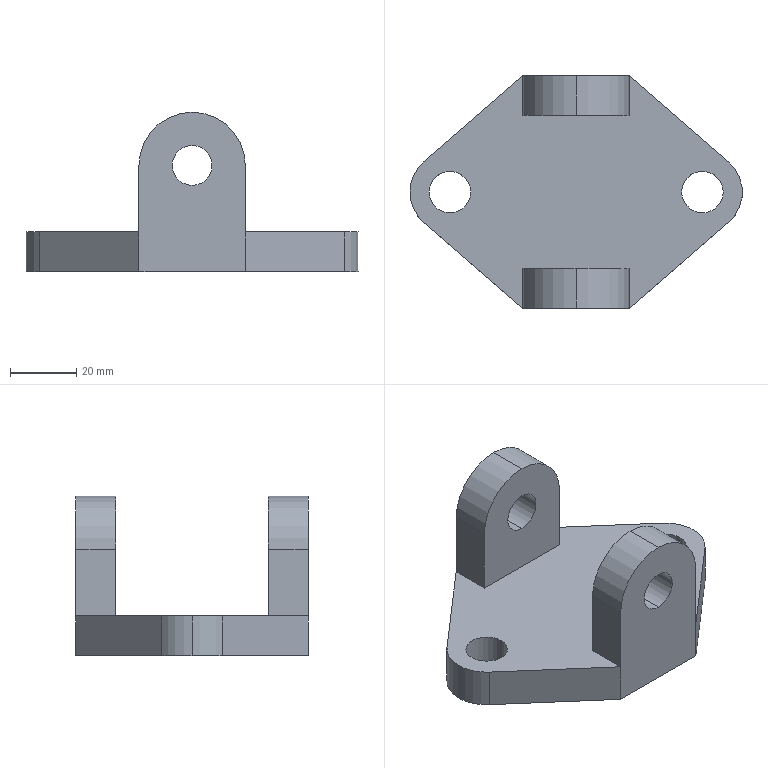Part | SolidWorks | features Cut 2, Boss 1, Extrusion 1, Fillet 1 | 1 solid | 29 faces | box 99.999 x 70 x 48 mm | volume 79061 mm3 | cylinder 15 | plane 14 | commonest cylinder face diameters 12 x4 12.5 x4 32 x4 24 x2 23.999 x1
STEP:
#1=CARTESIAN_POINT('',(0.,35.,38.));
#2=VERTEX_POINT('',#1);
#3=CARTESIAN_POINT('',(0.,35.,26.));
#4=VERTEX_POINT('',#3);
#5=CARTESIAN_POINT('',(0.,35.,32.));
#6=DIRECTION('',(0.,-1.,0.));
#7=DIRECTION('',(0.,0.,-1.));
#8=AXIS2_PLACEMENT_3D('',#5,#6,#7);
#9=CIRCLE('',#8,6.);
#10=EDGE_CURVE('',#2,#4,#9,.T.);
#11=ORIENTED_EDGE('',*,*,#10,.F.);
#12=CARTESIAN_POINT('',(0.,23.,38.));
#13=VERTEX_POINT('',#12);
#14=CARTESIAN_POINT('',(0.,43.,38.));
#15=DIRECTION('',(0.,-1.,0.));
#16=VECTOR('',#15,1000.);
#17=LINE('',#14,#16);
#18=EDGE_CURVE('',#2,#13,#17,.T.);
#19=ORIENTED_EDGE('',*,*,#18,.T.);
#20=CARTESIAN_POINT('',(0.,23.,26.));
#21=VERTEX_POINT('',#20);
#22=CARTESIAN_POINT('',(0.,23.,32.));
#23=DIRECTION('',(0.,1.,0.));
#24=DIRECTION('',(0.,0.,1.));
#25=AXIS2_PLACEMENT_3D('',#22,#23,#24);
#26=CIRCLE('',#25,6.);
#27=EDGE_CURVE('',#21,#13,#26,.T.);
#28=ORIENTED_EDGE('',*,*,#27,.F.);
#29=CARTESIAN_POINT('',(0.,43.,26.));
#30=DIRECTION('',(0.,-1.,0.));
#31=VECTOR('',#30,1000.);
#32=LINE('',#29,#31);
#33=EDGE_CURVE('',#4,#21,#32,.T.);
#34=ORIENTED_EDGE('',*,*,#33,.F.);
#35=EDGE_LOOP('',(#11,#19,#28,#34));
#36=FACE_OUTER_BOUND('',#35,.T.);
#37=CARTESIAN_POINT('',(0.,43.,32.));
#38=DIRECTION('',(0.,-1.,0.));
#39=DIRECTION('',(0.,0.,-1.));
#40=AXIS2_PLACEMENT_3D('',#37,#38,#39);
#41=CYLINDRICAL_SURFACE('',#40,6.);
#42=ADVANCED_FACE('',(#36),#41,.F.);
#43=CARTESIAN_POINT('',(0.,-23.,38.));
#44=VERTEX_POINT('',#43);
#45=CARTESIAN_POINT('',(0.,-23.,26.));
#46=VERTEX_POINT('',#45);
#47=CARTESIAN_POINT('',(0.,-23.,32.));
#48=DIRECTION('',(0.,-1.,0.));
#49=DIRECTION('',(0.,0.,-1.));
#50=AXIS2_PLACEMENT_3D('',#47,#48,#49);
#51=CIRCLE('',#50,6.);
#52=EDGE_CURVE('',#44,#46,#51,.T.);
#53=ORIENTED_EDGE('',*,*,#52,.F.);
#54=CARTESIAN_POINT('',(0.,-35.,38.));
#55=VERTEX_POINT('',#54);
#56=CARTESIAN_POINT('',(0.,43.,38.));
#57=DIRECTION('',(0.,-1.,0.));
#58=VECTOR('',#57,1000.);
#59=LINE('',#56,#58);
#60=EDGE_CURVE('',#44,#55,#59,.T.);
#61=ORIENTED_EDGE('',*,*,#60,.T.);
#62=CARTESIAN_POINT('',(0.,-35.,26.));
#63=VERTEX_POINT('',#62);
#64=CARTESIAN_POINT('',(0.,-35.,32.));
#65=DIRECTION('',(0.,-1.,0.));
#66=DIRECTION('',(0.,0.,-1.));
#67=AXIS2_PLACEMENT_3D('',#64,#65,#66);
#68=CIRCLE('',#67,6.);
#69=EDGE_CURVE('',#55,#63,#68,.T.);
#70=ORIENTED_EDGE('',*,*,#69,.T.);
#71=CARTESIAN_POINT('',(0.,43.,26.));
#72=DIRECTION('',(0.,-1.,0.));
#73=VECTOR('',#72,1000.);
#74=LINE('',#71,#73);
#75=EDGE_CURVE('',#46,#63,#74,.T.);
#76=ORIENTED_EDGE('',*,*,#75,.F.);
#77=EDGE_LOOP('',(#53,#61,#70,#76));
#78=FACE_OUTER_BOUND('',#77,.T.);
#79=CARTESIAN_POINT('',(0.,43.,32.));
#80=DIRECTION('',(0.,-1.,0.));
#81=DIRECTION('',(0.,0.,-1.));
#82=AXIS2_PLACEMENT_3D('',#79,#80,#81);
#83=CYLINDRICAL_SURFACE('',#82,6.);
#84=ADVANCED_FACE('',(#78),#83,.F.);
#85=CARTESIAN_POINT('',(31.75,0.,0.));
#86=VERTEX_POINT('',#85);
#87=CARTESIAN_POINT('',(44.25,0.,0.));
#88=VERTEX_POINT('',#87);
#89=CARTESIAN_POINT('',(38.,0.,0.));
#90=DIRECTION('',(0.,0.,1.));
#91=DIRECTION('',(1.,0.,0.));
#92=AXIS2_PLACEMENT_3D('',#89,#90,#91);
#93=CIRCLE('',#92,6.25);
#94=EDGE_CURVE('',#86,#88,#93,.T.);
#95=ORIENTED_EDGE('',*,*,#94,.F.);
#96=CARTESIAN_POINT('',(31.75,0.,12.));
#97=VERTEX_POINT('',#96);
#98=CARTESIAN_POINT('',(31.75,0.,0.));
#99=DIRECTION('',(0.,0.,1.));
#100=VECTOR('',#99,1000.);
#101=LINE('',#98,#100);
#102=EDGE_CURVE('',#86,#97,#101,.T.);
#103=ORIENTED_EDGE('',*,*,#102,.T.);
#104=CARTESIAN_POINT('',(44.25,0.,12.));
#105=VERTEX_POINT('',#104);
#106=CARTESIAN_POINT('',(38.,0.,12.));
#107=DIRECTION('',(0.,0.,1.));
#108=DIRECTION('',(1.,0.,0.));
#109=AXIS2_PLACEMENT_3D('',#106,#107,#108);
#110=CIRCLE('',#109,6.25);
#111=EDGE_CURVE('',#97,#105,#110,.T.);
#112=ORIENTED_EDGE('',*,*,#111,.T.);
#113=CARTESIAN_POINT('',(44.25,0.,0.));
#114=DIRECTION('',(0.,0.,1.));
#115=VECTOR('',#114,1000.);
#116=LINE('',#113,#115);
#117=EDGE_CURVE('',#88,#105,#116,.T.);
#118=ORIENTED_EDGE('',*,*,#117,.F.);
#119=EDGE_LOOP('',(#95,#103,#112,#118));
#120=FACE_OUTER_BOUND('',#119,.T.);
#121=CARTESIAN_POINT('',(38.,0.,0.));
#122=DIRECTION('',(0.,0.,1.));
#123=DIRECTION('',(1.,0.,0.));
#124=AXIS2_PLACEMENT_3D('',#121,#122,#123);
#125=CYLINDRICAL_SURFACE('',#124,6.25);
#126=ADVANCED_FACE('',(#120),#125,.F.);
#127=CARTESIAN_POINT('',(-44.25,0.,0.));
#128=VERTEX_POINT('',#127);
#129=CARTESIAN_POINT('',(-31.75,0.,0.));
#130=VERTEX_POINT('',#129);
#131=CARTESIAN_POINT('',(-38.,0.,0.));
#132=DIRECTION('',(0.,0.,1.));
#133=DIRECTION('',(1.,0.,0.));
#134=AXIS2_PLACEMENT_3D('',#131,#132,#133);
#135=CIRCLE('',#134,6.25);
#136=EDGE_CURVE('',#128,#130,#135,.T.);
#137=ORIENTED_EDGE('',*,*,#136,.F.);
#138=CARTESIAN_POINT('',(-44.25,0.,12.));
#139=VERTEX_POINT('',#138);
#140=CARTESIAN_POINT('',(-44.25,0.,0.));
#141=DIRECTION('',(0.,0.,1.));
#142=VECTOR('',#141,1000.);
#143=LINE('',#140,#142);
#144=EDGE_CURVE('',#128,#139,#143,.T.);
#145=ORIENTED_EDGE('',*,*,#144,.T.);
#146=CARTESIAN_POINT('',(-31.75,0.,12.));
#147=VERTEX_POINT('',#146);
#148=CARTESIAN_POINT('',(-38.,0.,12.));
#149=DIRECTION('',(0.,0.,1.));
#150=DIRECTION('',(1.,0.,0.));
#151=AXIS2_PLACEMENT_3D('',#148,#149,#150);
#152=CIRCLE('',#151,6.25);
#153=EDGE_CURVE('',#139,#147,#152,.T.);
#154=ORIENTED_EDGE('',*,*,#153,.T.);
#155=CARTESIAN_POINT('',(-31.75,0.,0.));
#156=DIRECTION('',(0.,0.,1.));
#157=VECTOR('',#156,1000.);
#158=LINE('',#155,#157);
#159=EDGE_CURVE('',#130,#147,#158,.T.);
#160=ORIENTED_EDGE('',*,*,#159,.F.);
#161=EDGE_LOOP('',(#137,#145,#154,#160));
#162=FACE_OUTER_BOUND('',#161,.T.);
#163=CARTESIAN_POINT('',(-38.,0.,0.));
#164=DIRECTION('',(0.,0.,1.));
#165=DIRECTION('',(1.,0.,0.));
#166=AXIS2_PLACEMENT_3D('',#163,#164,#165);
#167=CYLINDRICAL_SURFACE('',#166,6.25);
#168=ADVANCED_FACE('',(#162),#167,.F.);
#169=CARTESIAN_POINT('',(-50.,0.,12.));
#170=VERTEX_POINT('',#169);
#171=CARTESIAN_POINT('',(-45.868,-9.06,12.));
#172=VERTEX_POINT('',#171);
#173=CARTESIAN_POINT('',(-38.,0.,12.));
#174=DIRECTION('',(0.,0.,1.));
#175=DIRECTION('',(1.,0.,0.));
#176=AXIS2_PLACEMENT_3D('',#173,#174,#175);
#177=CIRCLE('',#176,12.);
#178=EDGE_CURVE('',#170,#172,#177,.T.);
#179=ORIENTED_EDGE('',*,*,#178,.F.);
#180=CARTESIAN_POINT('',(-50.,0.,0.));
#181=VERTEX_POINT('',#180);
#182=CARTESIAN_POINT('',(-50.,0.,12.));
#183=DIRECTION('',(0.,0.,-1.));
#184=VECTOR('',#183,1000.);
#185=LINE('',#182,#184);
#186=EDGE_CURVE('',#170,#181,#185,.T.);
#187=ORIENTED_EDGE('',*,*,#186,.T.);
#188=CARTESIAN_POINT('',(-45.868,-9.06,0.));
#189=VERTEX_POINT('',#188);
#190=CARTESIAN_POINT('',(-38.,0.,0.));
#191=DIRECTION('',(0.,0.,1.));
#192=DIRECTION('',(1.,0.,0.));
#193=AXIS2_PLACEMENT_3D('',#190,#191,#192);
#194=CIRCLE('',#193,12.);
#195=EDGE_CURVE('',#181,#189,#194,.T.);
#196=ORIENTED_EDGE('',*,*,#195,.T.);
#197=CARTESIAN_POINT('',(-45.868,-9.06,12.));
#198=DIRECTION('',(0.,0.,-1.));
#199=VECTOR('',#198,1000.);
#200=LINE('',#197,#199);
#201=EDGE_CURVE('',#172,#189,#200,.T.);
#202=ORIENTED_EDGE('',*,*,#201,.F.);
#203=EDGE_LOOP('',(#179,#187,#196,#202));
#204=FACE_OUTER_BOUND('',#203,.T.);
#205=CARTESIAN_POINT('',(-38.,0.,12.));
#206=DIRECTION('',(0.,0.,-1.));
#207=DIRECTION('',(-1.,0.,0.));
#208=AXIS2_PLACEMENT_3D('',#205,#206,#207);
#209=CYLINDRICAL_SURFACE('',#208,12.);
#210=ADVANCED_FACE('',(#204),#209,.T.);
#211=CARTESIAN_POINT('',(-38.,0.,12.));
#212=DIRECTION('',(0.,0.,1.));
#213=DIRECTION('',(1.,0.,0.));
#214=AXIS2_PLACEMENT_3D('',#211,#212,#213);
#215=CIRCLE('',#214,6.25);
#216=EDGE_CURVE('',#147,#139,#215,.T.);
#217=ORIENTED_EDGE('',*,*,#216,.F.);
#218=ORIENTED_EDGE('',*,*,#153,.F.);
#219=EDGE_LOOP('',(#217,#218));
#220=FACE_BOUND('',#219,.T.);
#221=CARTESIAN_POINT('',(38.,0.,12.));
#222=DIRECTION('',(0.,0.,1.));
#223=DIRECTION('',(1.,0.,0.));
#224=AXIS2_PLACEMENT_3D('',#221,#222,#223);
#225=CIRCLE('',#224,6.25);
#226=EDGE_CURVE('',#105,#97,#225,.T.);
#227=ORIENTED_EDGE('',*,*,#226,.F.);
#228=ORIENTED_EDGE('',*,*,#111,.F.);
#229=EDGE_LOOP('',(#227,#228));
#230=FACE_BOUND('',#229,.T.);
#231=CARTESIAN_POINT('',(-16.,-35.,12.));
#232=VERTEX_POINT('',#231);
#233=CARTESIAN_POINT('',(-16.,-35.,12.));
#234=DIRECTION('',(0.755,-0.6557,0.));
#235=VECTOR('',#234,1000.);
#236=LINE('',#233,#235);
#237=EDGE_CURVE('',#172,#232,#236,.T.);
#238=ORIENTED_EDGE('',*,*,#237,.T.);
#239=CARTESIAN_POINT('',(-16.,-23.,12.));
#240=VERTEX_POINT('',#239);
#241=CARTESIAN_POINT('',(-16.,-35.,12.));
#242=DIRECTION('',(0.,-1.,0.));
#243=VECTOR('',#242,1000.);
#244=LINE('',#241,#243);
#245=EDGE_CURVE('',#240,#232,#244,.T.);
#246=ORIENTED_EDGE('',*,*,#245,.F.);
#247=CARTESIAN_POINT('',(16.,-23.,12.));
#248=VERTEX_POINT('',#247);
#249=CARTESIAN_POINT('',(-16.,-23.,12.));
#250=DIRECTION('',(-1.,0.,0.));
#251=VECTOR('',#250,1000.);
#252=LINE('',#249,#251);
#253=EDGE_CURVE('',#248,#240,#252,.T.);
#254=ORIENTED_EDGE('',*,*,#253,.F.);
#255=CARTESIAN_POINT('',(16.,-35.,12.));
#256=VERTEX_POINT('',#255);
#257=CARTESIAN_POINT('',(16.,-35.,12.));
#258=DIRECTION('',(0.,1.,0.));
#259=VECTOR('',#258,1000.);
#260=LINE('',#257,#259);
#261=EDGE_CURVE('',#256,#248,#260,.T.);
#262=ORIENTED_EDGE('',*,*,#261,.F.);
#263=CARTESIAN_POINT('',(45.868,-9.06,12.));
#264=VERTEX_POINT('',#263);
#265=CARTESIAN_POINT('',(16.,-35.,12.));
#266=DIRECTION('',(0.755,0.6557,0.));
#267=VECTOR('',#266,1000.);
#268=LINE('',#265,#267);
#269=EDGE_CURVE('',#256,#264,#268,.T.);
#270=ORIENTED_EDGE('',*,*,#269,.T.);
#271=CARTESIAN_POINT('',(45.868,9.06,12.));
#272=VERTEX_POINT('',#271);
#273=CARTESIAN_POINT('',(38.,0.,12.));
#274=DIRECTION('',(0.,0.,1.));
#275=DIRECTION('',(1.,0.,0.));
#276=AXIS2_PLACEMENT_3D('',#273,#274,#275);
#277=CIRCLE('',#276,11.999);
#278=EDGE_CURVE('',#264,#272,#277,.T.);
#279=ORIENTED_EDGE('',*,*,#278,.T.);
#280=CARTESIAN_POINT('',(16.,35.,12.));
#281=VERTEX_POINT('',#280);
#282=CARTESIAN_POINT('',(16.,35.,12.));
#283=DIRECTION('',(-0.755,0.6557,0.));
#284=VECTOR('',#283,1000.);
#285=LINE('',#282,#284);
#286=EDGE_CURVE('',#272,#281,#285,.T.);
#287=ORIENTED_EDGE('',*,*,#286,.T.);
#288=CARTESIAN_POINT('',(16.,23.,12.));
#289=VERTEX_POINT('',#288);
#290=CARTESIAN_POINT('',(16.,35.,12.));
#291=DIRECTION('',(0.,1.,0.));
#292=VECTOR('',#291,1000.);
#293=LINE('',#290,#292);
#294=EDGE_CURVE('',#289,#281,#293,.T.);
#295=ORIENTED_EDGE('',*,*,#294,.F.);
#296=CARTESIAN_POINT('',(-16.,23.,12.));
#297=VERTEX_POINT('',#296);
#298=CARTESIAN_POINT('',(-16.,23.,12.));
#299=DIRECTION('',(1.,0.,0.));
#300=VECTOR('',#299,1000.);
#301=LINE('',#298,#300);
#302=EDGE_CURVE('',#297,#289,#301,.T.);
#303=ORIENTED_EDGE('',*,*,#302,.F.);
#304=CARTESIAN_POINT('',(-16.,35.,12.));
#305=VERTEX_POINT('',#304);
#306=CARTESIAN_POINT('',(-16.,35.,12.));
#307=DIRECTION('',(0.,-1.,0.));
#308=VECTOR('',#307,1000.);
#309=LINE('',#306,#308);
#310=EDGE_CURVE('',#305,#297,#309,.T.);
#311=ORIENTED_EDGE('',*,*,#310,.F.);
#312=CARTESIAN_POINT('',(-45.868,9.06,12.));
#313=VERTEX_POINT('',#312);
#314=CARTESIAN_POINT('',(-16.,35.,12.));
#315=DIRECTION('',(-0.755,-0.6557,0.));
#316=VECTOR('',#315,1000.);
#317=LINE('',#314,#316);
#318=EDGE_CURVE('',#305,#313,#317,.T.);
#319=ORIENTED_EDGE('',*,*,#318,.T.);
#320=CARTESIAN_POINT('',(-38.,0.,12.));
#321=DIRECTION('',(0.,0.,1.));
#322=DIRECTION('',(1.,0.,0.));
#323=AXIS2_PLACEMENT_3D('',#320,#321,#322);
#324=CIRCLE('',#323,12.);
#325=EDGE_CURVE('',#313,#170,#324,.T.);
#326=ORIENTED_EDGE('',*,*,#325,.T.);
#327=ORIENTED_EDGE('',*,*,#178,.T.);
#328=EDGE_LOOP('',(#238,#246,#254,#262,#270,#279,#287,#295,#303,#311,#319,#326,#327));
#329=FACE_OUTER_BOUND('',#328,.T.);
#330=CARTESIAN_POINT('',(38.,0.,12.));
#331=DIRECTION('',(0.,0.,1.));
#332=DIRECTION('',(1.,0.,0.));
#333=AXIS2_PLACEMENT_3D('',#330,#331,#332);
#334=PLANE('',#333);
#335=ADVANCED_FACE('',(#220,#230,#329),#334,.T.);
#336=CARTESIAN_POINT('',(0.,35.,32.));
#337=DIRECTION('',(0.,-1.,0.));
#338=DIRECTION('',(0.,0.,-1.));
#339=AXIS2_PLACEMENT_3D('',#336,#337,#338);
#340=CIRCLE('',#339,6.);
#341=EDGE_CURVE('',#4,#2,#340,.T.);
#342=ORIENTED_EDGE('',*,*,#341,.T.);
#343=ORIENTED_EDGE('',*,*,#10,.T.);
#344=EDGE_LOOP('',(#342,#343));
#345=FACE_BOUND('',#344,.T.);
#346=CARTESIAN_POINT('',(-16.,35.,32.));
#347=VERTEX_POINT('',#346);
#348=CARTESIAN_POINT('',(0.,35.,48.));
#349=VERTEX_POINT('',#348);
#350=CARTESIAN_POINT('',(0.,35.,32.));
#351=DIRECTION('',(0.,1.,0.));
#352=DIRECTION('',(0.,0.,-1.));
#353=AXIS2_PLACEMENT_3D('',#350,#351,#352);
#354=CIRCLE('',#353,16.);
#355=EDGE_CURVE('',#347,#349,#354,.T.);
#356=ORIENTED_EDGE('',*,*,#355,.T.);
#357=CARTESIAN_POINT('',(16.,35.,32.));
#358=VERTEX_POINT('',#357);
#359=CARTESIAN_POINT('',(0.,35.,32.));
#360=DIRECTION('',(0.,1.,0.));
#361=DIRECTION('',(0.,0.,-1.));
#362=AXIS2_PLACEMENT_3D('',#359,#360,#361);
#363=CIRCLE('',#362,16.);
#364=EDGE_CURVE('',#349,#358,#363,.T.);
#365=ORIENTED_EDGE('',*,*,#364,.T.);
#366=CARTESIAN_POINT('',(16.,35.,48.));
#367=DIRECTION('',(0.,0.,-1.));
#368=VECTOR('',#367,1000.);
#369=LINE('',#366,#368);
#370=EDGE_CURVE('',#358,#281,#369,.T.);
#371=ORIENTED_EDGE('',*,*,#370,.T.);
#372=CARTESIAN_POINT('',(16.,35.,0.));
#373=VERTEX_POINT('',#372);
#374=CARTESIAN_POINT('',(16.,35.,12.));
#375=DIRECTION('',(0.,0.,-1.));
#376=VECTOR('',#375,1000.);
#377=LINE('',#374,#376);
#378=EDGE_CURVE('',#281,#373,#377,.T.);
#379=ORIENTED_EDGE('',*,*,#378,.T.);
#380=CARTESIAN_POINT('',(-16.,35.,0.));
#381=VERTEX_POINT('',#380);
#382=CARTESIAN_POINT('',(0.,35.,0.));
#383=DIRECTION('',(-1.,0.,0.));
#384=VECTOR('',#383,1000.);
#385=LINE('',#382,#384);
#386=EDGE_CURVE('',#373,#381,#385,.T.);
#387=ORIENTED_EDGE('',*,*,#386,.T.);
#388=CARTESIAN_POINT('',(-16.,35.,12.));
#389=DIRECTION('',(0.,0.,-1.));
#390=VECTOR('',#389,1000.);
#391=LINE('',#388,#390);
#392=EDGE_CURVE('',#305,#381,#391,.T.);
#393=ORIENTED_EDGE('',*,*,#392,.F.);
#394=CARTESIAN_POINT('',(-16.,35.,48.));
#395=DIRECTION('',(0.,0.,-1.));
#396=VECTOR('',#395,1000.);
#397=LINE('',#394,#396);
#398=EDGE_CURVE('',#347,#305,#397,.T.);
#399=ORIENTED_EDGE('',*,*,#398,.F.);
#400=EDGE_LOOP('',(#356,#365,#371,#379,#387,#393,#399));
#401=FACE_OUTER_BOUND('',#400,.T.);
#402=CARTESIAN_POINT('',(0.,35.,12.));
#403=DIRECTION('',(0.,-1.,0.));
#404=DIRECTION('',(0.,0.,-1.));
#405=AXIS2_PLACEMENT_3D('',#402,#403,#404);
#406=PLANE('',#405);
#407=ADVANCED_FACE('',(#345,#401),#406,.F.);
#408=CARTESIAN_POINT('',(-45.868,9.06,0.));
#409=VERTEX_POINT('',#408);
#410=CARTESIAN_POINT('',(-16.,35.,0.));
#411=DIRECTION('',(-0.755,-0.6557,0.));
#412=VECTOR('',#411,1000.);
#413=LINE('',#410,#412);
#414=EDGE_CURVE('',#381,#409,#413,.T.);
#415=ORIENTED_EDGE('',*,*,#414,.T.);
#416=CARTESIAN_POINT('',(-45.868,9.06,12.));
#417=DIRECTION('',(0.,0.,-1.));
#418=VECTOR('',#417,1000.);
#419=LINE('',#416,#418);
#420=EDGE_CURVE('',#313,#409,#419,.T.);
#421=ORIENTED_EDGE('',*,*,#420,.F.);
#422=ORIENTED_EDGE('',*,*,#318,.F.);
#423=ORIENTED_EDGE('',*,*,#392,.T.);
#424=EDGE_LOOP('',(#415,#421,#422,#423));
#425=FACE_OUTER_BOUND('',#424,.T.);
#426=CARTESIAN_POINT('',(-16.,35.,12.));
#427=DIRECTION('',(0.6557,-0.755,0.));
#428=DIRECTION('',(0.755,0.6557,0.));
#429=AXIS2_PLACEMENT_3D('',#426,#427,#428);
#430=PLANE('',#429);
#431=ADVANCED_FACE('',(#425),#430,.F.);
#432=ORIENTED_EDGE('',*,*,#186,.F.);
#433=ORIENTED_EDGE('',*,*,#325,.F.);
#434=ORIENTED_EDGE('',*,*,#420,.T.);
#435=CARTESIAN_POINT('',(-38.,0.,0.));
#436=DIRECTION('',(0.,0.,1.));
#437=DIRECTION('',(1.,0.,0.));
#438=AXIS2_PLACEMENT_3D('',#435,#436,#437);
#439=CIRCLE('',#438,12.);
#440=EDGE_CURVE('',#409,#181,#439,.T.);
#441=ORIENTED_EDGE('',*,*,#440,.T.);
#442=EDGE_LOOP('',(#432,#433,#434,#441));
#443=FACE_OUTER_BOUND('',#442,.T.);
#444=CARTESIAN_POINT('',(-38.,0.,12.));
#445=DIRECTION('',(0.,0.,-1.));
#446=DIRECTION('',(-1.,0.,0.));
#447=AXIS2_PLACEMENT_3D('',#444,#445,#446);
#448=CYLINDRICAL_SURFACE('',#447,12.);
#449=ADVANCED_FACE('',(#443),#448,.T.);
#450=CARTESIAN_POINT('',(-16.,-35.,0.));
#451=VERTEX_POINT('',#450);
#452=CARTESIAN_POINT('',(-16.,-35.,0.));
#453=DIRECTION('',(0.755,-0.6557,0.));
#454=VECTOR('',#453,1000.);
#455=LINE('',#452,#454);
#456=EDGE_CURVE('',#189,#451,#455,.T.);
#457=ORIENTED_EDGE('',*,*,#456,.T.);
#458=CARTESIAN_POINT('',(-16.,-35.,12.));
#459=DIRECTION('',(0.,0.,-1.));
#460=VECTOR('',#459,1000.);
#461=LINE('',#458,#460);
#462=EDGE_CURVE('',#232,#451,#461,.T.);
#463=ORIENTED_EDGE('',*,*,#462,.F.);
#464=ORIENTED_EDGE('',*,*,#237,.F.);
#465=ORIENTED_EDGE('',*,*,#201,.T.);
#466=EDGE_LOOP('',(#457,#463,#464,#465));
#467=FACE_OUTER_BOUND('',#466,.T.);
#468=CARTESIAN_POINT('',(-16.,-35.,12.));
#469=DIRECTION('',(0.6557,0.755,0.));
#470=DIRECTION('',(-0.755,0.6557,0.));
#471=AXIS2_PLACEMENT_3D('',#468,#469,#470);
#472=PLANE('',#471);
#473=ADVANCED_FACE('',(#467),#472,.F.);
#474=CARTESIAN_POINT('',(0.,-35.,32.));
#475=DIRECTION('',(0.,-1.,0.));
#476=DIRECTION('',(0.,0.,-1.));
#477=AXIS2_PLACEMENT_3D('',#474,#475,#476);
#478=CIRCLE('',#477,6.);
#479=EDGE_CURVE('',#63,#55,#478,.T.);
#480=ORIENTED_EDGE('',*,*,#479,.F.);
#481=ORIENTED_EDGE('',*,*,#69,.F.);
#482=EDGE_LOOP('',(#480,#481));
#483=FACE_BOUND('',#482,.T.);
#484=CARTESIAN_POINT('',(16.,-35.,32.));
#485=VERTEX_POINT('',#484);
#486=CARTESIAN_POINT('',(16.,-35.,48.));
#487=DIRECTION('',(0.,0.,-1.));
#488=VECTOR('',#487,1000.);
#489=LINE('',#486,#488);
#490=EDGE_CURVE('',#485,#256,#489,.T.);
#491=ORIENTED_EDGE('',*,*,#490,.F.);
#492=CARTESIAN_POINT('',(0.,-35.,48.));
#493=VERTEX_POINT('',#492);
#494=CARTESIAN_POINT('',(0.,-35.,32.));
#495=DIRECTION('',(0.,-1.,0.));
#496=DIRECTION('',(0.,0.,1.));
#497=AXIS2_PLACEMENT_3D('',#494,#495,#496);
#498=CIRCLE('',#497,16.);
#499=EDGE_CURVE('',#485,#493,#498,.T.);
#500=ORIENTED_EDGE('',*,*,#499,.T.);
#501=CARTESIAN_POINT('',(-16.,-35.,32.));
#502=VERTEX_POINT('',#501);
#503=CARTESIAN_POINT('',(0.,-35.,32.));
#504=DIRECTION('',(0.,-1.,0.));
#505=DIRECTION('',(0.,0.,1.));
#506=AXIS2_PLACEMENT_3D('',#503,#504,#505);
#507=CIRCLE('',#506,16.);
#508=EDGE_CURVE('',#493,#502,#507,.T.);
#509=ORIENTED_EDGE('',*,*,#508,.T.);
#510=CARTESIAN_POINT('',(-16.,-35.,48.));
#511=DIRECTION('',(0.,0.,-1.));
#512=VECTOR('',#511,1000.);
#513=LINE('',#510,#512);
#514=EDGE_CURVE('',#502,#232,#513,.T.);
#515=ORIENTED_EDGE('',*,*,#514,.T.);
#516=ORIENTED_EDGE('',*,*,#462,.T.);
#517=CARTESIAN_POINT('',(16.,-35.,0.));
#518=VERTEX_POINT('',#517);
#519=CARTESIAN_POINT('',(-16.,-35.,0.));
#520=DIRECTION('',(1.,0.,0.));
#521=VECTOR('',#520,1000.);
#522=LINE('',#519,#521);
#523=EDGE_CURVE('',#451,#518,#522,.T.);
#524=ORIENTED_EDGE('',*,*,#523,.T.);
#525=CARTESIAN_POINT('',(16.,-35.,12.));
#526=DIRECTION('',(0.,0.,-1.));
#527=VECTOR('',#526,1000.);
#528=LINE('',#525,#527);
#529=EDGE_CURVE('',#256,#518,#528,.T.);
#530=ORIENTED_EDGE('',*,*,#529,.F.);
#531=EDGE_LOOP('',(#491,#500,#509,#515,#516,#524,#530));
#532=FACE_OUTER_BOUND('',#531,.T.);
#533=CARTESIAN_POINT('',(-16.,-35.,12.));
#534=DIRECTION('',(0.,1.,0.));
#535=DIRECTION('',(0.,0.,1.));
#536=AXIS2_PLACEMENT_3D('',#533,#534,#535);
#537=PLANE('',#536);
#538=ADVANCED_FACE('',(#483,#532),#537,.F.);
#539=CARTESIAN_POINT('',(45.868,-9.06,0.));
#540=VERTEX_POINT('',#539);
#541=CARTESIAN_POINT('',(16.,-35.,0.));
#542=DIRECTION('',(0.755,0.6557,0.));
#543=VECTOR('',#542,1000.);
#544=LINE('',#541,#543);
#545=EDGE_CURVE('',#518,#540,#544,.T.);
#546=ORIENTED_EDGE('',*,*,#545,.T.);
#547=CARTESIAN_POINT('',(45.868,-9.06,12.));
#548=DIRECTION('',(0.,0.,-1.));
#549=VECTOR('',#548,1000.);
#550=LINE('',#547,#549);
#551=EDGE_CURVE('',#264,#540,#550,.T.);
#552=ORIENTED_EDGE('',*,*,#551,.F.);
#553=ORIENTED_EDGE('',*,*,#269,.F.);
#554=ORIENTED_EDGE('',*,*,#529,.T.);
#555=EDGE_LOOP('',(#546,#552,#553,#554));
#556=FACE_OUTER_BOUND('',#555,.T.);
#557=CARTESIAN_POINT('',(16.,-35.,12.));
#558=DIRECTION('',(-0.6557,0.755,0.));
#559=DIRECTION('',(-0.755,-0.6557,0.));
#560=AXIS2_PLACEMENT_3D('',#557,#558,#559);
#561=PLANE('',#560);
#562=ADVANCED_FACE('',(#556),#561,.F.);
#563=CARTESIAN_POINT('',(45.868,9.06,0.));
#564=VERTEX_POINT('',#563);
#565=CARTESIAN_POINT('',(38.,0.,0.));
#566=DIRECTION('',(0.,0.,1.));
#567=DIRECTION('',(1.,0.,0.));
#568=AXIS2_PLACEMENT_3D('',#565,#566,#567);
#569=CIRCLE('',#568,11.999);
#570=EDGE_CURVE('',#540,#564,#569,.T.);
#571=ORIENTED_EDGE('',*,*,#570,.T.);
#572=CARTESIAN_POINT('',(45.868,9.06,12.));
#573=DIRECTION('',(0.,0.,-1.));
#574=VECTOR('',#573,1000.);
#575=LINE('',#572,#574);
#576=EDGE_CURVE('',#272,#564,#575,.T.);
#577=ORIENTED_EDGE('',*,*,#576,.F.);
#578=ORIENTED_EDGE('',*,*,#278,.F.);
#579=ORIENTED_EDGE('',*,*,#551,.T.);
#580=EDGE_LOOP('',(#571,#577,#578,#579));
#581=FACE_OUTER_BOUND('',#580,.T.);
#582=CARTESIAN_POINT('',(38.,0.,12.));
#583=DIRECTION('',(0.,0.,-1.));
#584=DIRECTION('',(-1.,0.,0.));
#585=AXIS2_PLACEMENT_3D('',#582,#583,#584);
#586=CYLINDRICAL_SURFACE('',#585,11.999);
#587=ADVANCED_FACE('',(#581),#586,.T.);
#588=CARTESIAN_POINT('',(16.,35.,0.));
#589=DIRECTION('',(-0.755,0.6557,0.));
#590=VECTOR('',#589,1000.);
#591=LINE('',#588,#590);
#592=EDGE_CURVE('',#564,#373,#591,.T.);
#593=ORIENTED_EDGE('',*,*,#592,.T.);
#594=ORIENTED_EDGE('',*,*,#378,.F.);
#595=ORIENTED_EDGE('',*,*,#286,.F.);
#596=ORIENTED_EDGE('',*,*,#576,.T.);
#597=EDGE_LOOP('',(#593,#594,#595,#596));
#598=FACE_OUTER_BOUND('',#597,.T.);
#599=CARTESIAN_POINT('',(16.,35.,12.));
#600=DIRECTION('',(-0.6557,-0.755,0.));
#601=DIRECTION('',(0.755,-0.6557,0.));
#602=AXIS2_PLACEMENT_3D('',#599,#600,#601);
#603=PLANE('',#602);
#604=ADVANCED_FACE('',(#598),#603,.F.);
#605=CARTESIAN_POINT('',(38.,0.,0.));
#606=DIRECTION('',(0.,0.,1.));
#607=DIRECTION('',(1.,0.,0.));
#608=AXIS2_PLACEMENT_3D('',#605,#606,#607);
#609=CIRCLE('',#608,6.25);
#610=EDGE_CURVE('',#88,#86,#609,.T.);
#611=ORIENTED_EDGE('',*,*,#610,.T.);
#612=ORIENTED_EDGE('',*,*,#94,.T.);
#613=EDGE_LOOP('',(#611,#612));
#614=FACE_BOUND('',#613,.T.);
#615=CARTESIAN_POINT('',(-38.,0.,0.));
#616=DIRECTION('',(0.,0.,1.));
#617=DIRECTION('',(1.,0.,0.));
#618=AXIS2_PLACEMENT_3D('',#615,#616,#617);
#619=CIRCLE('',#618,6.25);
#620=EDGE_CURVE('',#130,#128,#619,.T.);
#621=ORIENTED_EDGE('',*,*,#620,.T.);
#622=ORIENTED_EDGE('',*,*,#136,.T.);
#623=EDGE_LOOP('',(#621,#622));
#624=FACE_BOUND('',#623,.T.);
#625=ORIENTED_EDGE('',*,*,#386,.F.);
#626=ORIENTED_EDGE('',*,*,#592,.F.);
#627=ORIENTED_EDGE('',*,*,#570,.F.);
#628=ORIENTED_EDGE('',*,*,#545,.F.);
#629=ORIENTED_EDGE('',*,*,#523,.F.);
#630=ORIENTED_EDGE('',*,*,#456,.F.);
#631=ORIENTED_EDGE('',*,*,#195,.F.);
#632=ORIENTED_EDGE('',*,*,#440,.F.);
#633=ORIENTED_EDGE('',*,*,#414,.F.);
#634=EDGE_LOOP('',(#625,#626,#627,#628,#629,#630,#631,#632,#633));
#635=FACE_OUTER_BOUND('',#634,.T.);
#636=CARTESIAN_POINT('',(38.,0.,0.));
#637=DIRECTION('',(0.,0.,1.));
#638=DIRECTION('',(1.,0.,0.));
#639=AXIS2_PLACEMENT_3D('',#636,#637,#638);
#640=PLANE('',#639);
#641=ADVANCED_FACE('',(#614,#624,#635),#640,.F.);
#642=ORIENTED_EDGE('',*,*,#144,.F.);
#643=ORIENTED_EDGE('',*,*,#620,.F.);
#644=ORIENTED_EDGE('',*,*,#159,.T.);
#645=ORIENTED_EDGE('',*,*,#216,.T.);
#646=EDGE_LOOP('',(#642,#643,#644,#645));
#647=FACE_OUTER_BOUND('',#646,.T.);
#648=CARTESIAN_POINT('',(-38.,0.,0.));
#649=DIRECTION('',(0.,0.,1.));
#650=DIRECTION('',(1.,0.,0.));
#651=AXIS2_PLACEMENT_3D('',#648,#649,#650);
#652=CYLINDRICAL_SURFACE('',#651,6.25);
#653=ADVANCED_FACE('',(#647),#652,.F.);
#654=ORIENTED_EDGE('',*,*,#102,.F.);
#655=ORIENTED_EDGE('',*,*,#610,.F.);
#656=ORIENTED_EDGE('',*,*,#117,.T.);
#657=ORIENTED_EDGE('',*,*,#226,.T.);
#658=EDGE_LOOP('',(#654,#655,#656,#657));
#659=FACE_OUTER_BOUND('',#658,.T.);
#660=CARTESIAN_POINT('',(38.,0.,0.));
#661=DIRECTION('',(0.,0.,1.));
#662=DIRECTION('',(1.,0.,0.));
#663=AXIS2_PLACEMENT_3D('',#660,#661,#662);
#664=CYLINDRICAL_SURFACE('',#663,6.25);
#665=ADVANCED_FACE('',(#659),#664,.F.);
#666=CARTESIAN_POINT('',(-16.,23.,32.));
#667=VERTEX_POINT('',#666);
#668=CARTESIAN_POINT('',(-16.,23.,48.));
#669=DIRECTION('',(0.,0.,-1.));
#670=VECTOR('',#669,1000.);
#671=LINE('',#668,#670);
#672=EDGE_CURVE('',#667,#297,#671,.T.);
#673=ORIENTED_EDGE('',*,*,#672,.F.);
#674=CARTESIAN_POINT('',(-16.,35.,32.));
#675=DIRECTION('',(0.,1.,0.));
#676=VECTOR('',#675,1000.);
#677=LINE('',#674,#676);
#678=EDGE_CURVE('',#667,#347,#677,.T.);
#679=ORIENTED_EDGE('',*,*,#678,.T.);
#680=ORIENTED_EDGE('',*,*,#398,.T.);
#681=ORIENTED_EDGE('',*,*,#310,.T.);
#682=EDGE_LOOP('',(#673,#679,#680,#681));
#683=FACE_OUTER_BOUND('',#682,.T.);
#684=CARTESIAN_POINT('',(-16.,35.,48.));
#685=DIRECTION('',(1.,0.,0.));
#686=DIRECTION('',(0.,0.,-1.));
#687=AXIS2_PLACEMENT_3D('',#684,#685,#686);
#688=PLANE('',#687);
#689=ADVANCED_FACE('',(#683),#688,.F.);
#690=ORIENTED_EDGE('',*,*,#27,.T.);
#691=CARTESIAN_POINT('',(0.,23.,32.));
#692=DIRECTION('',(0.,1.,0.));
#693=DIRECTION('',(0.,0.,1.));
#694=AXIS2_PLACEMENT_3D('',#691,#692,#693);
#695=CIRCLE('',#694,6.);
#696=EDGE_CURVE('',#13,#21,#695,.T.);
#697=ORIENTED_EDGE('',*,*,#696,.T.);
#698=EDGE_LOOP('',(#690,#697));
#699=FACE_BOUND('',#698,.T.);
#700=CARTESIAN_POINT('',(16.,23.,32.));
#701=VERTEX_POINT('',#700);
#702=CARTESIAN_POINT('',(16.,23.,48.));
#703=DIRECTION('',(0.,0.,-1.));
#704=VECTOR('',#703,1000.);
#705=LINE('',#702,#704);
#706=EDGE_CURVE('',#701,#289,#705,.T.);
#707=ORIENTED_EDGE('',*,*,#706,.F.);
#708=CARTESIAN_POINT('',(0.,23.,48.));
#709=VERTEX_POINT('',#708);
#710=CARTESIAN_POINT('',(0.,23.,32.));
#711=DIRECTION('',(0.,-1.,0.));
#712=DIRECTION('',(0.,0.,1.));
#713=AXIS2_PLACEMENT_3D('',#710,#711,#712);
#714=CIRCLE('',#713,16.);
#715=EDGE_CURVE('',#701,#709,#714,.T.);
#716=ORIENTED_EDGE('',*,*,#715,.T.);
#717=CARTESIAN_POINT('',(0.,23.,32.));
#718=DIRECTION('',(0.,-1.,0.));
#719=DIRECTION('',(0.,0.,1.));
#720=AXIS2_PLACEMENT_3D('',#717,#718,#719);
#721=CIRCLE('',#720,16.);
#722=EDGE_CURVE('',#709,#667,#721,.T.);
#723=ORIENTED_EDGE('',*,*,#722,.T.);
#724=ORIENTED_EDGE('',*,*,#672,.T.);
#725=ORIENTED_EDGE('',*,*,#302,.T.);
#726=EDGE_LOOP('',(#707,#716,#723,#724,#725));
#727=FACE_OUTER_BOUND('',#726,.T.);
#728=CARTESIAN_POINT('',(-16.,23.,48.));
#729=DIRECTION('',(0.,1.,0.));
#730=DIRECTION('',(0.,0.,1.));
#731=AXIS2_PLACEMENT_3D('',#728,#729,#730);
#732=PLANE('',#731);
#733=ADVANCED_FACE('',(#699,#727),#732,.F.);
#734=ORIENTED_EDGE('',*,*,#370,.F.);
#735=CARTESIAN_POINT('',(16.,23.,32.));
#736=DIRECTION('',(0.,-1.,0.));
#737=VECTOR('',#736,1000.);
#738=LINE('',#735,#737);
#739=EDGE_CURVE('',#358,#701,#738,.T.);
#740=ORIENTED_EDGE('',*,*,#739,.T.);
#741=ORIENTED_EDGE('',*,*,#706,.T.);
#742=ORIENTED_EDGE('',*,*,#294,.T.);
#743=EDGE_LOOP('',(#734,#740,#741,#742));
#744=FACE_OUTER_BOUND('',#743,.T.);
#745=CARTESIAN_POINT('',(16.,35.,48.));
#746=DIRECTION('',(-1.,0.,0.));
#747=DIRECTION('',(0.,0.,1.));
#748=AXIS2_PLACEMENT_3D('',#745,#746,#747);
#749=PLANE('',#748);
#750=ADVANCED_FACE('',(#744),#749,.F.);
#751=ORIENTED_EDGE('',*,*,#514,.F.);
#752=CARTESIAN_POINT('',(-16.,-23.,32.));
#753=VERTEX_POINT('',#752);
#754=CARTESIAN_POINT('',(-16.,-35.,32.));
#755=DIRECTION('',(0.,1.,0.));
#756=VECTOR('',#755,1000.);
#757=LINE('',#754,#756);
#758=EDGE_CURVE('',#502,#753,#757,.T.);
#759=ORIENTED_EDGE('',*,*,#758,.T.);
#760=CARTESIAN_POINT('',(-16.,-23.,48.));
#761=DIRECTION('',(0.,0.,-1.));
#762=VECTOR('',#761,1000.);
#763=LINE('',#760,#762);
#764=EDGE_CURVE('',#753,#240,#763,.T.);
#765=ORIENTED_EDGE('',*,*,#764,.T.);
#766=ORIENTED_EDGE('',*,*,#245,.T.);
#767=EDGE_LOOP('',(#751,#759,#765,#766));
#768=FACE_OUTER_BOUND('',#767,.T.);
#769=CARTESIAN_POINT('',(-16.,-35.,48.));
#770=DIRECTION('',(1.,0.,0.));
#771=DIRECTION('',(0.,0.,-1.));
#772=AXIS2_PLACEMENT_3D('',#769,#770,#771);
#773=PLANE('',#772);
#774=ADVANCED_FACE('',(#768),#773,.F.);
#775=CARTESIAN_POINT('',(16.,-23.,32.));
#776=VERTEX_POINT('',#775);
#777=CARTESIAN_POINT('',(16.,-23.,48.));
#778=DIRECTION('',(0.,0.,-1.));
#779=VECTOR('',#778,1000.);
#780=LINE('',#777,#779);
#781=EDGE_CURVE('',#776,#248,#780,.T.);
#782=ORIENTED_EDGE('',*,*,#781,.F.);
#783=CARTESIAN_POINT('',(16.,-35.,32.));
#784=DIRECTION('',(0.,-1.,0.));
#785=VECTOR('',#784,1000.);
#786=LINE('',#783,#785);
#787=EDGE_CURVE('',#776,#485,#786,.T.);
#788=ORIENTED_EDGE('',*,*,#787,.T.);
#789=ORIENTED_EDGE('',*,*,#490,.T.);
#790=ORIENTED_EDGE('',*,*,#261,.T.);
#791=EDGE_LOOP('',(#782,#788,#789,#790));
#792=FACE_OUTER_BOUND('',#791,.T.);
#793=CARTESIAN_POINT('',(16.,-35.,48.));
#794=DIRECTION('',(-1.,0.,0.));
#795=DIRECTION('',(0.,0.,1.));
#796=AXIS2_PLACEMENT_3D('',#793,#794,#795);
#797=PLANE('',#796);
#798=ADVANCED_FACE('',(#792),#797,.F.);
#799=CARTESIAN_POINT('',(0.,-23.,32.));
#800=DIRECTION('',(0.,-1.,0.));
#801=DIRECTION('',(0.,0.,-1.));
#802=AXIS2_PLACEMENT_3D('',#799,#800,#801);
#803=CIRCLE('',#802,6.);
#804=EDGE_CURVE('',#46,#44,#803,.T.);
#805=ORIENTED_EDGE('',*,*,#804,.T.);
#806=ORIENTED_EDGE('',*,*,#52,.T.);
#807=EDGE_LOOP('',(#805,#806));
#808=FACE_BOUND('',#807,.T.);
#809=CARTESIAN_POINT('',(0.,-23.,48.));
#810=VERTEX_POINT('',#809);
#811=CARTESIAN_POINT('',(0.,-23.,32.));
#812=DIRECTION('',(0.,1.,0.));
#813=DIRECTION('',(0.,0.,-1.));
#814=AXIS2_PLACEMENT_3D('',#811,#812,#813);
#815=CIRCLE('',#814,16.);
#816=EDGE_CURVE('',#753,#810,#815,.T.);
#817=ORIENTED_EDGE('',*,*,#816,.T.);
#818=CARTESIAN_POINT('',(0.,-23.,32.));
#819=DIRECTION('',(0.,1.,0.));
#820=DIRECTION('',(0.,0.,-1.));
#821=AXIS2_PLACEMENT_3D('',#818,#819,#820);
#822=CIRCLE('',#821,16.);
#823=EDGE_CURVE('',#810,#776,#822,.T.);
#824=ORIENTED_EDGE('',*,*,#823,.T.);
#825=ORIENTED_EDGE('',*,*,#781,.T.);
#826=ORIENTED_EDGE('',*,*,#253,.T.);
#827=ORIENTED_EDGE('',*,*,#764,.F.);
#828=EDGE_LOOP('',(#817,#824,#825,#826,#827));
#829=FACE_OUTER_BOUND('',#828,.T.);
#830=CARTESIAN_POINT('',(-16.,-23.,48.));
#831=DIRECTION('',(0.,-1.,0.));
#832=DIRECTION('',(0.,0.,-1.));
#833=AXIS2_PLACEMENT_3D('',#830,#831,#832);
#834=PLANE('',#833);
#835=ADVANCED_FACE('',(#808,#829),#834,.F.);
#836=ORIENTED_EDGE('',*,*,#60,.F.);
#837=ORIENTED_EDGE('',*,*,#804,.F.);
#838=ORIENTED_EDGE('',*,*,#75,.T.);
#839=ORIENTED_EDGE('',*,*,#479,.T.);
#840=EDGE_LOOP('',(#836,#837,#838,#839));
#841=FACE_OUTER_BOUND('',#840,.T.);
#842=CARTESIAN_POINT('',(0.,43.,32.));
#843=DIRECTION('',(0.,-1.,0.));
#844=DIRECTION('',(0.,0.,-1.));
#845=AXIS2_PLACEMENT_3D('',#842,#843,#844);
#846=CYLINDRICAL_SURFACE('',#845,6.);
#847=ADVANCED_FACE('',(#841),#846,.F.);
#848=ORIENTED_EDGE('',*,*,#18,.F.);
#849=ORIENTED_EDGE('',*,*,#341,.F.);
#850=ORIENTED_EDGE('',*,*,#33,.T.);
#851=ORIENTED_EDGE('',*,*,#696,.F.);
#852=EDGE_LOOP('',(#848,#849,#850,#851));
#853=FACE_OUTER_BOUND('',#852,.T.);
#854=CARTESIAN_POINT('',(0.,43.,32.));
#855=DIRECTION('',(0.,-1.,0.));
#856=DIRECTION('',(0.,0.,-1.));
#857=AXIS2_PLACEMENT_3D('',#854,#855,#856);
#858=CYLINDRICAL_SURFACE('',#857,6.);
#859=ADVANCED_FACE('',(#853),#858,.F.);
#860=ORIENTED_EDGE('',*,*,#678,.F.);
#861=ORIENTED_EDGE('',*,*,#722,.F.);
#862=CARTESIAN_POINT('',(0.,23.,48.));
#863=DIRECTION('',(0.,-1.,0.));
#864=VECTOR('',#863,1000.);
#865=LINE('',#862,#864);
#866=EDGE_CURVE('',#349,#709,#865,.T.);
#867=ORIENTED_EDGE('',*,*,#866,.F.);
#868=ORIENTED_EDGE('',*,*,#355,.F.);
#869=EDGE_LOOP('',(#860,#861,#867,#868));
#870=FACE_OUTER_BOUND('',#869,.T.);
#871=CARTESIAN_POINT('',(0.,23.,32.));
#872=DIRECTION('',(0.,1.,0.));
#873=DIRECTION('',(0.,0.,1.));
#874=AXIS2_PLACEMENT_3D('',#871,#872,#873);
#875=CYLINDRICAL_SURFACE('',#874,16.);
#876=ADVANCED_FACE('',(#870),#875,.T.);
#877=ORIENTED_EDGE('',*,*,#715,.F.);
#878=ORIENTED_EDGE('',*,*,#739,.F.);
#879=ORIENTED_EDGE('',*,*,#364,.F.);
#880=ORIENTED_EDGE('',*,*,#866,.T.);
#881=EDGE_LOOP('',(#877,#878,#879,#880));
#882=FACE_OUTER_BOUND('',#881,.T.);
#883=CARTESIAN_POINT('',(0.,23.,32.));
#884=DIRECTION('',(0.,-1.,0.));
#885=DIRECTION('',(0.,0.,-1.));
#886=AXIS2_PLACEMENT_3D('',#883,#884,#885);
#887=CYLINDRICAL_SURFACE('',#886,16.);
#888=ADVANCED_FACE('',(#882),#887,.T.);
#889=ORIENTED_EDGE('',*,*,#758,.F.);
#890=ORIENTED_EDGE('',*,*,#508,.F.);
#891=CARTESIAN_POINT('',(0.,-23.,48.));
#892=DIRECTION('',(0.,-1.,0.));
#893=VECTOR('',#892,1000.);
#894=LINE('',#891,#893);
#895=EDGE_CURVE('',#810,#493,#894,.T.);
#896=ORIENTED_EDGE('',*,*,#895,.F.);
#897=ORIENTED_EDGE('',*,*,#816,.F.);
#898=EDGE_LOOP('',(#889,#890,#896,#897));
#899=FACE_OUTER_BOUND('',#898,.T.);
#900=CARTESIAN_POINT('',(0.,-23.,32.));
#901=DIRECTION('',(0.,-1.,0.));
#902=DIRECTION('',(0.,0.,-1.));
#903=AXIS2_PLACEMENT_3D('',#900,#901,#902);
#904=CYLINDRICAL_SURFACE('',#903,16.);
#905=ADVANCED_FACE('',(#899),#904,.T.);
#906=ORIENTED_EDGE('',*,*,#499,.F.);
#907=ORIENTED_EDGE('',*,*,#787,.F.);
#908=ORIENTED_EDGE('',*,*,#823,.F.);
#909=ORIENTED_EDGE('',*,*,#895,.T.);
#910=EDGE_LOOP('',(#906,#907,#908,#909));
#911=FACE_OUTER_BOUND('',#910,.T.);
#912=CARTESIAN_POINT('',(0.,-23.,32.));
#913=DIRECTION('',(0.,1.,0.));
#914=DIRECTION('',(0.,0.,1.));
#915=AXIS2_PLACEMENT_3D('',#912,#913,#914);
#916=CYLINDRICAL_SURFACE('',#915,16.);
#917=ADVANCED_FACE('',(#911),#916,.T.);
#918=CLOSED_SHELL('',(#42,#84,#126,#168,#210,#335,#407,#431,#449,#473,#538,#562,#587,#604,#641,#653,#665,#689,#733,#750,#774,#798,#835,#847,#859,#876,#888,#905,#917));
#919=MANIFOLD_SOLID_BREP('',#918);
#920=CARTESIAN_POINT('',(0.,0.,0.));
#921=DIRECTION('',(0.,0.,1.));
#922=DIRECTION('',(1.,0.,0.));
#923=AXIS2_PLACEMENT_3D('',#920,#921,#922);
#924=(LENGTH_UNIT()NAMED_UNIT(*)SI_UNIT(.MILLI.,.METRE.));
#925=UNCERTAINTY_MEASURE_WITH_UNIT(LENGTH_MEASURE(0.00001),#924,'','');
#926=(NAMED_UNIT(*)PLANE_ANGLE_UNIT()SI_UNIT($,.RADIAN.));
#927=(NAMED_UNIT(*)SI_UNIT($,.STERADIAN.)SOLID_ANGLE_UNIT());
#928=(GEOMETRIC_REPRESENTATION_CONTEXT(3)GLOBAL_UNCERTAINTY_ASSIGNED_CONTEXT((#925))GLOBAL_UNIT_ASSIGNED_CONTEXT((#924,#926,#927))REPRESENTATION_CONTEXT('',''));
#929=ADVANCED_BREP_SHAPE_REPRESENTATION('',(#919,#923),#928);